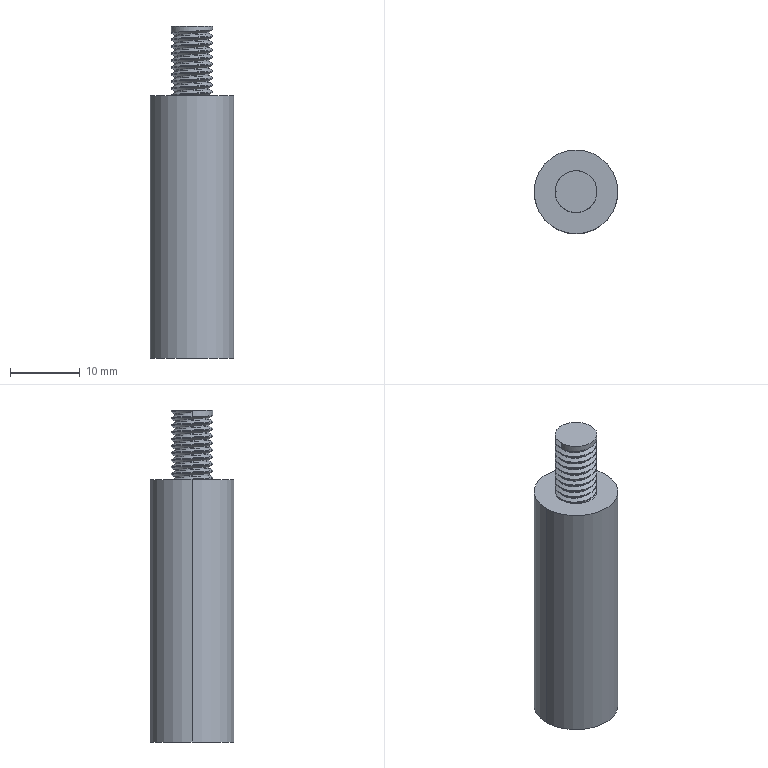Part | NX | features BREP 1 | 1 solid | 36 faces | box 12 x 12 x 47.5 mm | volume 4380 mm3 | cylinder 27 | plane 5 | cone 2 | spline 2 | commonest cylinder face diameters 6 x22 3.3 x2 12 x2 4.917 x1